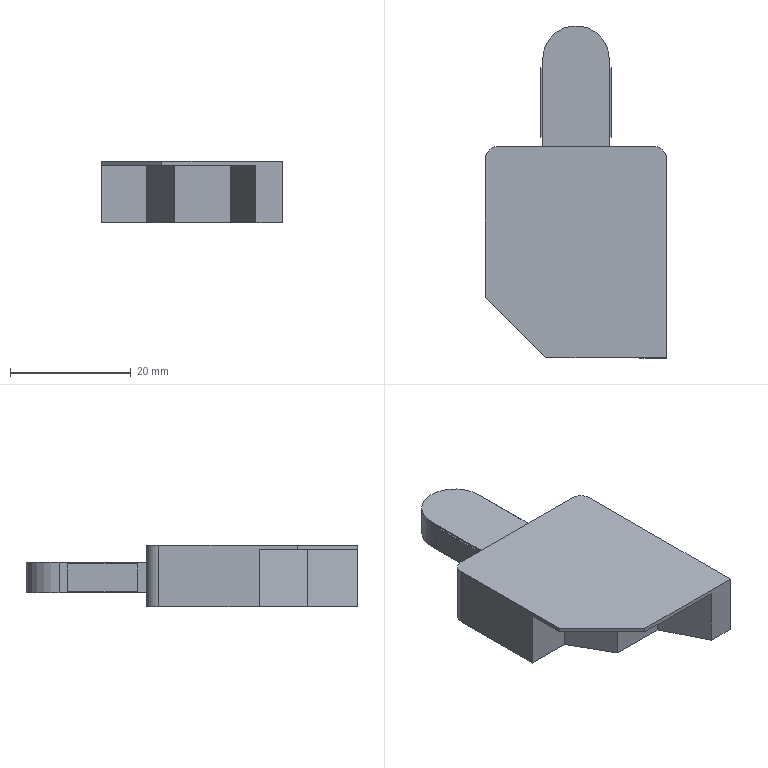Part | SolidWorks | features BaseBody 1 | 1 solid | 29 faces | box 30 x 55 x 10.2 mm | volume 9110 mm3 | plane 26 | cylinder 3 | commonest cylinder face diameters 4 x2 11 x1
STEP:
#1=CARTESIAN_POINT('',(244.946,-4065.971,2034.471));
#2=VERTEX_POINT('',#1);
#3=CARTESIAN_POINT('',(244.946,-4042.971,2034.471));
#4=VERTEX_POINT('',#3);
#5=CARTESIAN_POINT('',(244.946,-4075.971,2034.471));
#6=DIRECTION('',(0.,1.,0.));
#7=VECTOR('',#6,1000.);
#8=LINE('',#5,#7);
#9=EDGE_CURVE('',#2,#4,#8,.T.);
#10=ORIENTED_EDGE('',*,*,#9,.F.);
#11=CARTESIAN_POINT('',(254.946,-4075.971,2034.471));
#12=VERTEX_POINT('',#11);
#13=CARTESIAN_POINT('',(254.946,-4075.971,2034.471));
#14=DIRECTION('',(-0.7071,0.7071,0.));
#15=VECTOR('',#14,1000.);
#16=LINE('',#13,#15);
#17=EDGE_CURVE('',#12,#2,#16,.T.);
#18=ORIENTED_EDGE('',*,*,#17,.F.);
#19=CARTESIAN_POINT('',(274.946,-4075.971,2034.471));
#20=VERTEX_POINT('',#19);
#21=CARTESIAN_POINT('',(254.946,-4075.971,2034.471));
#22=DIRECTION('',(-1.,0.,0.));
#23=VECTOR('',#22,1000.);
#24=LINE('',#21,#23);
#25=EDGE_CURVE('',#20,#12,#24,.T.);
#26=ORIENTED_EDGE('',*,*,#25,.F.);
#27=CARTESIAN_POINT('',(274.946,-4042.971,2034.471));
#28=VERTEX_POINT('',#27);
#29=CARTESIAN_POINT('',(274.946,-4075.971,2034.471));
#30=DIRECTION('',(0.,-1.,0.));
#31=VECTOR('',#30,1000.);
#32=LINE('',#29,#31);
#33=EDGE_CURVE('',#28,#20,#32,.T.);
#34=ORIENTED_EDGE('',*,*,#33,.F.);
#35=CARTESIAN_POINT('',(272.946,-4040.971,2034.471));
#36=VERTEX_POINT('',#35);
#37=CARTESIAN_POINT('',(272.946,-4042.971,2034.471));
#38=DIRECTION('',(0.,0.,-1.));
#39=DIRECTION('',(1.,0.,0.));
#40=AXIS2_PLACEMENT_3D('',#37,#38,#39);
#41=CIRCLE('',#40,2.);
#42=EDGE_CURVE('',#36,#28,#41,.T.);
#43=ORIENTED_EDGE('',*,*,#42,.F.);
#44=CARTESIAN_POINT('',(246.946,-4040.971,2034.471));
#45=VERTEX_POINT('',#44);
#46=CARTESIAN_POINT('',(254.946,-4040.971,2034.471));
#47=DIRECTION('',(1.,0.,0.));
#48=VECTOR('',#47,1000.);
#49=LINE('',#46,#48);
#50=EDGE_CURVE('',#45,#36,#49,.T.);
#51=ORIENTED_EDGE('',*,*,#50,.F.);
#52=CARTESIAN_POINT('',(246.946,-4042.971,2034.471));
#53=DIRECTION('',(0.,0.,-1.));
#54=DIRECTION('',(1.,0.,0.));
#55=AXIS2_PLACEMENT_3D('',#52,#53,#54);
#56=CIRCLE('',#55,2.);
#57=EDGE_CURVE('',#4,#45,#56,.T.);
#58=ORIENTED_EDGE('',*,*,#57,.F.);
#59=EDGE_LOOP('',(#10,#18,#26,#34,#43,#51,#58));
#60=FACE_OUTER_BOUND('',#59,.T.);
#61=CARTESIAN_POINT('',(254.946,-4075.971,2034.471));
#62=DIRECTION('',(0.,0.,-1.));
#63=DIRECTION('',(-1.,0.,0.));
#64=AXIS2_PLACEMENT_3D('',#61,#62,#63);
#65=PLANE('',#64);
#66=ADVANCED_FACE('',(#60),#65,.F.);
#67=CARTESIAN_POINT('',(244.946,-4042.971,2024.271));
#68=VERTEX_POINT('',#67);
#69=CARTESIAN_POINT('',(244.946,-4042.971,2033.771));
#70=DIRECTION('',(0.,0.,1.));
#71=VECTOR('',#70,1000.);
#72=LINE('',#69,#71);
#73=EDGE_CURVE('',#68,#4,#72,.T.);
#74=ORIENTED_EDGE('',*,*,#73,.T.);
#75=ORIENTED_EDGE('',*,*,#57,.T.);
#76=CARTESIAN_POINT('',(246.946,-4040.971,2024.271));
#77=VERTEX_POINT('',#76);
#78=CARTESIAN_POINT('',(246.946,-4040.971,2033.771));
#79=DIRECTION('',(0.,0.,-1.));
#80=VECTOR('',#79,1000.);
#81=LINE('',#78,#80);
#82=EDGE_CURVE('',#45,#77,#81,.T.);
#83=ORIENTED_EDGE('',*,*,#82,.T.);
#84=CARTESIAN_POINT('',(246.946,-4042.971,2024.271));
#85=DIRECTION('',(0.,0.,1.));
#86=DIRECTION('',(1.,0.,0.));
#87=AXIS2_PLACEMENT_3D('',#84,#85,#86);
#88=CIRCLE('',#87,2.);
#89=EDGE_CURVE('',#77,#68,#88,.T.);
#90=ORIENTED_EDGE('',*,*,#89,.T.);
#91=EDGE_LOOP('',(#74,#75,#83,#90));
#92=FACE_OUTER_BOUND('',#91,.T.);
#93=CARTESIAN_POINT('',(246.946,-4042.971,2033.771));
#94=DIRECTION('',(0.,0.,1.));
#95=DIRECTION('',(1.,0.,0.));
#96=AXIS2_PLACEMENT_3D('',#93,#94,#95);
#97=CYLINDRICAL_SURFACE('',#96,2.);
#98=ADVANCED_FACE('',(#92),#97,.T.);
#99=CARTESIAN_POINT('',(244.946,-4065.971,2033.771));
#100=VERTEX_POINT('',#99);
#101=CARTESIAN_POINT('',(244.946,-4065.971,2033.771));
#102=DIRECTION('',(0.,0.,1.));
#103=VECTOR('',#102,1000.);
#104=LINE('',#101,#103);
#105=EDGE_CURVE('',#100,#2,#104,.T.);
#106=ORIENTED_EDGE('',*,*,#105,.T.);
#107=ORIENTED_EDGE('',*,*,#9,.T.);
#108=ORIENTED_EDGE('',*,*,#73,.F.);
#109=CARTESIAN_POINT('',(244.946,-4059.609,2024.271));
#110=VERTEX_POINT('',#109);
#111=CARTESIAN_POINT('',(244.946,-4065.971,2024.271));
#112=DIRECTION('',(0.,-1.,0.));
#113=VECTOR('',#112,1000.);
#114=LINE('',#111,#113);
#115=EDGE_CURVE('',#68,#110,#114,.T.);
#116=ORIENTED_EDGE('',*,*,#115,.T.);
#117=CARTESIAN_POINT('',(244.946,-4059.609,2033.771));
#118=VERTEX_POINT('',#117);
#119=CARTESIAN_POINT('',(244.946,-4059.609,2033.771));
#120=DIRECTION('',(0.,0.,1.));
#121=VECTOR('',#120,1000.);
#122=LINE('',#119,#121);
#123=EDGE_CURVE('',#110,#118,#122,.T.);
#124=ORIENTED_EDGE('',*,*,#123,.T.);
#125=CARTESIAN_POINT('',(244.946,-4065.971,2033.771));
#126=DIRECTION('',(0.,-1.,0.));
#127=VECTOR('',#126,1000.);
#128=LINE('',#125,#127);
#129=EDGE_CURVE('',#118,#100,#128,.T.);
#130=ORIENTED_EDGE('',*,*,#129,.T.);
#131=EDGE_LOOP('',(#106,#107,#108,#116,#124,#130));
#132=FACE_OUTER_BOUND('',#131,.T.);
#133=CARTESIAN_POINT('',(244.946,-4065.971,2033.771));
#134=DIRECTION('',(-1.,0.,0.));
#135=DIRECTION('',(0.,0.,1.));
#136=AXIS2_PLACEMENT_3D('',#133,#134,#135);
#137=PLANE('',#136);
#138=ADVANCED_FACE('',(#132),#137,.T.);
#139=CARTESIAN_POINT('',(254.946,-4075.971,2033.771));
#140=VERTEX_POINT('',#139);
#141=CARTESIAN_POINT('',(254.946,-4075.971,2033.771));
#142=DIRECTION('',(0.7071,-0.7071,0.));
#143=VECTOR('',#142,1000.);
#144=LINE('',#141,#143);
#145=EDGE_CURVE('',#100,#140,#144,.T.);
#146=ORIENTED_EDGE('',*,*,#145,.T.);
#147=CARTESIAN_POINT('',(254.946,-4075.971,2033.771));
#148=DIRECTION('',(0.,0.,1.));
#149=VECTOR('',#148,1000.);
#150=LINE('',#147,#149);
#151=EDGE_CURVE('',#140,#12,#150,.T.);
#152=ORIENTED_EDGE('',*,*,#151,.T.);
#153=ORIENTED_EDGE('',*,*,#17,.T.);
#154=ORIENTED_EDGE('',*,*,#105,.F.);
#155=EDGE_LOOP('',(#146,#152,#153,#154));
#156=FACE_OUTER_BOUND('',#155,.T.);
#157=CARTESIAN_POINT('',(254.946,-4075.971,2033.771));
#158=DIRECTION('',(-0.7071,-0.7071,0.));
#159=DIRECTION('',(0.7071,-0.7071,0.));
#160=AXIS2_PLACEMENT_3D('',#157,#158,#159);
#161=PLANE('',#160);
#162=ADVANCED_FACE('',(#156),#161,.T.);
#163=CARTESIAN_POINT('',(270.521,-4075.971,2024.271));
#164=VERTEX_POINT('',#163);
#165=CARTESIAN_POINT('',(274.946,-4075.971,2024.271));
#166=VERTEX_POINT('',#165);
#167=CARTESIAN_POINT('',(274.946,-4075.971,2024.271));
#168=DIRECTION('',(1.,0.,0.));
#169=VECTOR('',#168,1000.);
#170=LINE('',#167,#169);
#171=EDGE_CURVE('',#164,#166,#170,.T.);
#172=ORIENTED_EDGE('',*,*,#171,.T.);
#173=CARTESIAN_POINT('',(274.946,-4075.971,2033.771));
#174=DIRECTION('',(0.,0.,1.));
#175=VECTOR('',#174,1000.);
#176=LINE('',#173,#175);
#177=EDGE_CURVE('',#166,#20,#176,.T.);
#178=ORIENTED_EDGE('',*,*,#177,.T.);
#179=ORIENTED_EDGE('',*,*,#25,.T.);
#180=ORIENTED_EDGE('',*,*,#151,.F.);
#181=CARTESIAN_POINT('',(270.521,-4075.971,2033.771));
#182=VERTEX_POINT('',#181);
#183=CARTESIAN_POINT('',(274.946,-4075.971,2033.771));
#184=DIRECTION('',(1.,0.,0.));
#185=VECTOR('',#184,1000.);
#186=LINE('',#183,#185);
#187=EDGE_CURVE('',#140,#182,#186,.T.);
#188=ORIENTED_EDGE('',*,*,#187,.T.);
#189=CARTESIAN_POINT('',(270.521,-4075.971,2033.771));
#190=DIRECTION('',(0.,0.,-1.));
#191=VECTOR('',#190,1000.);
#192=LINE('',#189,#191);
#193=EDGE_CURVE('',#182,#164,#192,.T.);
#194=ORIENTED_EDGE('',*,*,#193,.T.);
#195=EDGE_LOOP('',(#172,#178,#179,#180,#188,#194));
#196=FACE_OUTER_BOUND('',#195,.T.);
#197=CARTESIAN_POINT('',(274.946,-4075.971,2033.771));
#198=DIRECTION('',(0.,-1.,0.));
#199=DIRECTION('',(0.,0.,-1.));
#200=AXIS2_PLACEMENT_3D('',#197,#198,#199);
#201=PLANE('',#200);
#202=ADVANCED_FACE('',(#196),#201,.T.);
#203=ORIENTED_EDGE('',*,*,#177,.F.);
#204=CARTESIAN_POINT('',(274.946,-4042.971,2024.271));
#205=VERTEX_POINT('',#204);
#206=CARTESIAN_POINT('',(274.946,-4040.971,2024.271));
#207=DIRECTION('',(0.,1.,0.));
#208=VECTOR('',#207,1000.);
#209=LINE('',#206,#208);
#210=EDGE_CURVE('',#166,#205,#209,.T.);
#211=ORIENTED_EDGE('',*,*,#210,.T.);
#212=CARTESIAN_POINT('',(274.946,-4042.971,2033.771));
#213=DIRECTION('',(0.,0.,1.));
#214=VECTOR('',#213,1000.);
#215=LINE('',#212,#214);
#216=EDGE_CURVE('',#205,#28,#215,.T.);
#217=ORIENTED_EDGE('',*,*,#216,.T.);
#218=ORIENTED_EDGE('',*,*,#33,.T.);
#219=EDGE_LOOP('',(#203,#211,#217,#218));
#220=FACE_OUTER_BOUND('',#219,.T.);
#221=CARTESIAN_POINT('',(274.946,-4040.971,2033.771));
#222=DIRECTION('',(1.,0.,0.));
#223=DIRECTION('',(0.,0.,-1.));
#224=AXIS2_PLACEMENT_3D('',#221,#222,#223);
#225=PLANE('',#224);
#226=ADVANCED_FACE('',(#220),#225,.T.);
#227=CARTESIAN_POINT('',(272.946,-4040.971,2024.271));
#228=VERTEX_POINT('',#227);
#229=CARTESIAN_POINT('',(272.946,-4040.971,2033.771));
#230=DIRECTION('',(0.,0.,1.));
#231=VECTOR('',#230,1000.);
#232=LINE('',#229,#231);
#233=EDGE_CURVE('',#228,#36,#232,.T.);
#234=ORIENTED_EDGE('',*,*,#233,.T.);
#235=ORIENTED_EDGE('',*,*,#42,.T.);
#236=ORIENTED_EDGE('',*,*,#216,.F.);
#237=CARTESIAN_POINT('',(272.946,-4042.971,2024.271));
#238=DIRECTION('',(0.,0.,1.));
#239=DIRECTION('',(1.,0.,0.));
#240=AXIS2_PLACEMENT_3D('',#237,#238,#239);
#241=CIRCLE('',#240,2.);
#242=EDGE_CURVE('',#205,#228,#241,.T.);
#243=ORIENTED_EDGE('',*,*,#242,.T.);
#244=EDGE_LOOP('',(#234,#235,#236,#243));
#245=FACE_OUTER_BOUND('',#244,.T.);
#246=CARTESIAN_POINT('',(272.946,-4042.971,2033.771));
#247=DIRECTION('',(0.,0.,1.));
#248=DIRECTION('',(1.,0.,0.));
#249=AXIS2_PLACEMENT_3D('',#246,#247,#248);
#250=CYLINDRICAL_SURFACE('',#249,2.);
#251=ADVANCED_FACE('',(#245),#250,.T.);
#252=ORIENTED_EDGE('',*,*,#233,.F.);
#253=CARTESIAN_POINT('',(244.946,-4040.971,2024.271));
#254=DIRECTION('',(-1.,0.,0.));
#255=VECTOR('',#254,1000.);
#256=LINE('',#253,#255);
#257=EDGE_CURVE('',#228,#77,#256,.T.);
#258=ORIENTED_EDGE('',*,*,#257,.T.);
#259=ORIENTED_EDGE('',*,*,#82,.F.);
#260=ORIENTED_EDGE('',*,*,#50,.T.);
#261=EDGE_LOOP('',(#252,#258,#259,#260));
#262=FACE_OUTER_BOUND('',#261,.T.);
#263=CARTESIAN_POINT('',(254.446,-4040.971,2031.613));
#264=VERTEX_POINT('',#263);
#265=CARTESIAN_POINT('',(254.446,-4040.971,2026.613));
#266=VERTEX_POINT('',#265);
#267=CARTESIAN_POINT('',(254.446,-4040.971,2033.771));
#268=DIRECTION('',(0.,0.,-1.));
#269=VECTOR('',#268,1000.);
#270=LINE('',#267,#269);
#271=EDGE_CURVE('',#264,#266,#270,.T.);
#272=ORIENTED_EDGE('',*,*,#271,.T.);
#273=CARTESIAN_POINT('',(265.446,-4040.971,2026.613));
#274=VERTEX_POINT('',#273);
#275=CARTESIAN_POINT('',(244.946,-4040.971,2026.613));
#276=DIRECTION('',(1.,0.,0.));
#277=VECTOR('',#276,1000.);
#278=LINE('',#275,#277);
#279=EDGE_CURVE('',#266,#274,#278,.T.);
#280=ORIENTED_EDGE('',*,*,#279,.T.);
#281=CARTESIAN_POINT('',(265.446,-4040.971,2031.613));
#282=VERTEX_POINT('',#281);
#283=CARTESIAN_POINT('',(265.446,-4040.971,2033.771));
#284=DIRECTION('',(0.,0.,1.));
#285=VECTOR('',#284,1000.);
#286=LINE('',#283,#285);
#287=EDGE_CURVE('',#274,#282,#286,.T.);
#288=ORIENTED_EDGE('',*,*,#287,.T.);
#289=CARTESIAN_POINT('',(244.946,-4040.971,2031.613));
#290=DIRECTION('',(-1.,0.,0.));
#291=VECTOR('',#290,1000.);
#292=LINE('',#289,#291);
#293=EDGE_CURVE('',#282,#264,#292,.T.);
#294=ORIENTED_EDGE('',*,*,#293,.T.);
#295=EDGE_LOOP('',(#272,#280,#288,#294));
#296=FACE_BOUND('',#295,.T.);
#297=CARTESIAN_POINT('',(244.946,-4040.971,2033.771));
#298=DIRECTION('',(0.,1.,0.));
#299=DIRECTION('',(0.,0.,1.));
#300=AXIS2_PLACEMENT_3D('',#297,#298,#299);
#301=PLANE('',#300);
#302=ADVANCED_FACE('',(#262,#296),#301,.T.);
#303=CARTESIAN_POINT('',(252.478,-4059.609,2024.271));
#304=VERTEX_POINT('',#303);
#305=CARTESIAN_POINT('',(260.766,-4059.609,2024.271));
#306=DIRECTION('',(-1.,0.,0.));
#307=VECTOR('',#306,1000.);
#308=LINE('',#305,#307);
#309=EDGE_CURVE('',#304,#110,#308,.T.);
#310=ORIENTED_EDGE('',*,*,#309,.T.);
#311=ORIENTED_EDGE('',*,*,#115,.F.);
#312=ORIENTED_EDGE('',*,*,#89,.F.);
#313=ORIENTED_EDGE('',*,*,#257,.F.);
#314=ORIENTED_EDGE('',*,*,#242,.F.);
#315=ORIENTED_EDGE('',*,*,#210,.F.);
#316=ORIENTED_EDGE('',*,*,#171,.F.);
#317=CARTESIAN_POINT('',(266.357,-4067.585,2024.271));
#318=VERTEX_POINT('',#317);
#319=CARTESIAN_POINT('',(270.521,-4075.971,2024.271));
#320=DIRECTION('',(-0.4447,0.8957,0.));
#321=VECTOR('',#320,1000.);
#322=LINE('',#319,#321);
#323=EDGE_CURVE('',#164,#318,#322,.T.);
#324=ORIENTED_EDGE('',*,*,#323,.T.);
#325=CARTESIAN_POINT('',(256.989,-4067.585,2024.271));
#326=VERTEX_POINT('',#325);
#327=CARTESIAN_POINT('',(260.766,-4067.585,2024.271));
#328=DIRECTION('',(-1.,0.,0.));
#329=VECTOR('',#328,1000.);
#330=LINE('',#327,#329);
#331=EDGE_CURVE('',#318,#326,#330,.T.);
#332=ORIENTED_EDGE('',*,*,#331,.T.);
#333=CARTESIAN_POINT('',(256.989,-4067.585,2024.271));
#334=DIRECTION('',(-0.4923,0.8704,0.));
#335=VECTOR('',#334,1000.);
#336=LINE('',#333,#335);
#337=EDGE_CURVE('',#326,#304,#336,.T.);
#338=ORIENTED_EDGE('',*,*,#337,.T.);
#339=EDGE_LOOP('',(#310,#311,#312,#313,#314,#315,#316,#324,#332,#338));
#340=FACE_OUTER_BOUND('',#339,.T.);
#341=CARTESIAN_POINT('',(260.766,-4061.034,2024.271));
#342=DIRECTION('',(0.,0.,-1.));
#343=DIRECTION('',(-1.,0.,0.));
#344=AXIS2_PLACEMENT_3D('',#341,#342,#343);
#345=PLANE('',#344);
#346=ADVANCED_FACE('',(#340),#345,.T.);
#347=ORIENTED_EDGE('',*,*,#145,.F.);
#348=ORIENTED_EDGE('',*,*,#129,.F.);
#349=CARTESIAN_POINT('',(252.478,-4059.609,2033.771));
#350=VERTEX_POINT('',#349);
#351=CARTESIAN_POINT('',(258.946,-4059.609,2033.771));
#352=DIRECTION('',(1.,0.,0.));
#353=VECTOR('',#352,1000.);
#354=LINE('',#351,#353);
#355=EDGE_CURVE('',#118,#350,#354,.T.);
#356=ORIENTED_EDGE('',*,*,#355,.T.);
#357=CARTESIAN_POINT('',(256.989,-4067.585,2033.771));
#358=VERTEX_POINT('',#357);
#359=CARTESIAN_POINT('',(252.478,-4059.609,2033.771));
#360=DIRECTION('',(0.4923,-0.8704,0.));
#361=VECTOR('',#360,1000.);
#362=LINE('',#359,#361);
#363=EDGE_CURVE('',#350,#358,#362,.T.);
#364=ORIENTED_EDGE('',*,*,#363,.T.);
#365=CARTESIAN_POINT('',(266.357,-4067.585,2033.771));
#366=VERTEX_POINT('',#365);
#367=CARTESIAN_POINT('',(258.946,-4067.585,2033.771));
#368=DIRECTION('',(1.,0.,0.));
#369=VECTOR('',#368,1000.);
#370=LINE('',#367,#369);
#371=EDGE_CURVE('',#358,#366,#370,.T.);
#372=ORIENTED_EDGE('',*,*,#371,.T.);
#373=CARTESIAN_POINT('',(266.357,-4067.585,2033.771));
#374=DIRECTION('',(0.4447,-0.8957,0.));
#375=VECTOR('',#374,1000.);
#376=LINE('',#373,#375);
#377=EDGE_CURVE('',#366,#182,#376,.T.);
#378=ORIENTED_EDGE('',*,*,#377,.T.);
#379=ORIENTED_EDGE('',*,*,#187,.F.);
#380=EDGE_LOOP('',(#347,#348,#356,#364,#372,#378,#379));
#381=FACE_OUTER_BOUND('',#380,.T.);
#382=CARTESIAN_POINT('',(258.946,-4059.971,2033.771));
#383=DIRECTION('',(0.,0.,-1.));
#384=DIRECTION('',(-1.,0.,0.));
#385=AXIS2_PLACEMENT_3D('',#382,#383,#384);
#386=PLANE('',#385);
#387=ADVANCED_FACE('',(#381),#386,.T.);
#388=ORIENTED_EDGE('',*,*,#309,.F.);
#389=CARTESIAN_POINT('',(252.478,-4059.609,2024.271));
#390=DIRECTION('',(0.,0.,1.));
#391=VECTOR('',#390,1000.);
#392=LINE('',#389,#391);
#393=EDGE_CURVE('',#304,#350,#392,.T.);
#394=ORIENTED_EDGE('',*,*,#393,.T.);
#395=ORIENTED_EDGE('',*,*,#355,.F.);
#396=ORIENTED_EDGE('',*,*,#123,.F.);
#397=EDGE_LOOP('',(#388,#394,#395,#396));
#398=FACE_OUTER_BOUND('',#397,.T.);
#399=CARTESIAN_POINT('',(252.478,-4059.609,2024.271));
#400=DIRECTION('',(0.,-1.,0.));
#401=DIRECTION('',(0.,0.,-1.));
#402=AXIS2_PLACEMENT_3D('',#399,#400,#401);
#403=PLANE('',#402);
#404=ADVANCED_FACE('',(#398),#403,.T.);
#405=ORIENTED_EDGE('',*,*,#323,.F.);
#406=ORIENTED_EDGE('',*,*,#193,.F.);
#407=ORIENTED_EDGE('',*,*,#377,.F.);
#408=CARTESIAN_POINT('',(266.357,-4067.585,2024.271));
#409=DIRECTION('',(0.,0.,-1.));
#410=VECTOR('',#409,1000.);
#411=LINE('',#408,#410);
#412=EDGE_CURVE('',#366,#318,#411,.T.);
#413=ORIENTED_EDGE('',*,*,#412,.T.);
#414=EDGE_LOOP('',(#405,#406,#407,#413));
#415=FACE_OUTER_BOUND('',#414,.T.);
#416=CARTESIAN_POINT('',(270.521,-4075.971,2024.271));
#417=DIRECTION('',(-0.8957,-0.4447,0.));
#418=DIRECTION('',(0.4447,-0.8957,0.));
#419=AXIS2_PLACEMENT_3D('',#416,#417,#418);
#420=PLANE('',#419);
#421=ADVANCED_FACE('',(#415),#420,.T.);
#422=CARTESIAN_POINT('',(265.446,-4026.471,2026.613));
#423=VERTEX_POINT('',#422);
#424=CARTESIAN_POINT('',(265.446,-4006.471,2026.613));
#425=DIRECTION('',(0.,1.,0.));
#426=VECTOR('',#425,1000.);
#427=LINE('',#424,#426);
#428=EDGE_CURVE('',#274,#423,#427,.T.);
#429=ORIENTED_EDGE('',*,*,#428,.F.);
#430=ORIENTED_EDGE('',*,*,#279,.F.);
#431=CARTESIAN_POINT('',(254.446,-4026.471,2026.613));
#432=VERTEX_POINT('',#431);
#433=CARTESIAN_POINT('',(254.446,-4006.471,2026.613));
#434=DIRECTION('',(0.,-1.,0.));
#435=VECTOR('',#434,1000.);
#436=LINE('',#433,#435);
#437=EDGE_CURVE('',#432,#266,#436,.T.);
#438=ORIENTED_EDGE('',*,*,#437,.F.);
#439=CARTESIAN_POINT('',(259.946,-4026.471,2026.613));
#440=DIRECTION('',(0.,0.,1.));
#441=DIRECTION('',(-1.,0.,0.));
#442=AXIS2_PLACEMENT_3D('',#439,#440,#441);
#443=CIRCLE('',#442,5.5);
#444=EDGE_CURVE('',#423,#432,#443,.T.);
#445=ORIENTED_EDGE('',*,*,#444,.F.);
#446=EDGE_LOOP('',(#429,#430,#438,#445));
#447=FACE_OUTER_BOUND('',#446,.T.);
#448=CARTESIAN_POINT('',(265.446,-4006.471,2026.613));
#449=DIRECTION('',(0.,0.,1.));
#450=DIRECTION('',(0.,-1.,0.));
#451=AXIS2_PLACEMENT_3D('',#448,#449,#450);
#452=PLANE('',#451);
#453=ADVANCED_FACE('',(#447),#452,.F.);
#454=CARTESIAN_POINT('',(254.446,-4027.908,2026.863));
#455=VERTEX_POINT('',#454);
#456=CARTESIAN_POINT('',(254.446,-4027.908,2031.363));
#457=VERTEX_POINT('',#456);
#458=CARTESIAN_POINT('',(254.446,-4027.908,2031.613));
#459=DIRECTION('',(0.,0.,1.));
#460=VECTOR('',#459,1000.);
#461=LINE('',#458,#460);
#462=EDGE_CURVE('',#455,#457,#461,.T.);
#463=ORIENTED_EDGE('',*,*,#462,.T.);
#464=CARTESIAN_POINT('',(254.446,-4039.428,2031.363));
#465=VERTEX_POINT('',#464);
#466=CARTESIAN_POINT('',(254.446,-4006.471,2031.363));
#467=DIRECTION('',(0.,-1.,0.));
#468=VECTOR('',#467,1000.);
#469=LINE('',#466,#468);
#470=EDGE_CURVE('',#457,#465,#469,.T.);
#471=ORIENTED_EDGE('',*,*,#470,.T.);
#472=CARTESIAN_POINT('',(254.446,-4039.428,2026.863));
#473=VERTEX_POINT('',#472);
#474=CARTESIAN_POINT('',(254.446,-4039.428,2031.613));
#475=DIRECTION('',(0.,0.,-1.));
#476=VECTOR('',#475,1000.);
#477=LINE('',#474,#476);
#478=EDGE_CURVE('',#465,#473,#477,.T.);
#479=ORIENTED_EDGE('',*,*,#478,.T.);
#480=CARTESIAN_POINT('',(254.446,-4006.471,2026.863));
#481=DIRECTION('',(0.,1.,0.));
#482=VECTOR('',#481,1000.);
#483=LINE('',#480,#482);
#484=EDGE_CURVE('',#473,#455,#483,.T.);
#485=ORIENTED_EDGE('',*,*,#484,.T.);
#486=EDGE_LOOP('',(#463,#471,#479,#485));
#487=FACE_BOUND('',#486,.T.);
#488=CARTESIAN_POINT('',(254.446,-4026.471,2031.613));
#489=VERTEX_POINT('',#488);
#490=CARTESIAN_POINT('',(254.446,-4006.471,2031.613));
#491=DIRECTION('',(0.,1.,0.));
#492=VECTOR('',#491,1000.);
#493=LINE('',#490,#492);
#494=EDGE_CURVE('',#264,#489,#493,.T.);
#495=ORIENTED_EDGE('',*,*,#494,.T.);
#496=CARTESIAN_POINT('',(254.446,-4026.471,2031.613));
#497=DIRECTION('',(0.,0.,-1.));
#498=VECTOR('',#497,1000.);
#499=LINE('',#496,#498);
#500=EDGE_CURVE('',#489,#432,#499,.T.);
#501=ORIENTED_EDGE('',*,*,#500,.T.);
#502=ORIENTED_EDGE('',*,*,#437,.T.);
#503=ORIENTED_EDGE('',*,*,#271,.F.);
#504=EDGE_LOOP('',(#495,#501,#502,#503));
#505=FACE_OUTER_BOUND('',#504,.T.);
#506=CARTESIAN_POINT('',(254.446,-4006.471,2031.613));
#507=DIRECTION('',(-1.,0.,0.));
#508=DIRECTION('',(0.,0.,1.));
#509=AXIS2_PLACEMENT_3D('',#506,#507,#508);
#510=PLANE('',#509);
#511=ADVANCED_FACE('',(#487,#505),#510,.T.);
#512=ORIENTED_EDGE('',*,*,#494,.F.);
#513=ORIENTED_EDGE('',*,*,#293,.F.);
#514=CARTESIAN_POINT('',(265.446,-4026.471,2031.613));
#515=VERTEX_POINT('',#514);
#516=CARTESIAN_POINT('',(265.446,-4014.431,2031.613));
#517=DIRECTION('',(0.,1.,0.));
#518=VECTOR('',#517,1000.);
#519=LINE('',#516,#518);
#520=EDGE_CURVE('',#282,#515,#519,.T.);
#521=ORIENTED_EDGE('',*,*,#520,.T.);
#522=CARTESIAN_POINT('',(259.946,-4026.471,2031.613));
#523=DIRECTION('',(0.,0.,1.));
#524=DIRECTION('',(-1.,0.,0.));
#525=AXIS2_PLACEMENT_3D('',#522,#523,#524);
#526=CIRCLE('',#525,5.5);
#527=EDGE_CURVE('',#515,#489,#526,.T.);
#528=ORIENTED_EDGE('',*,*,#527,.T.);
#529=EDGE_LOOP('',(#512,#513,#521,#528));
#530=FACE_OUTER_BOUND('',#529,.T.);
#531=CARTESIAN_POINT('',(259.946,-4014.431,2031.613));
#532=DIRECTION('',(0.,0.,1.));
#533=DIRECTION('',(0.,-1.,0.));
#534=AXIS2_PLACEMENT_3D('',#531,#532,#533);
#535=PLANE('',#534);
#536=ADVANCED_FACE('',(#530),#535,.T.);
#537=CARTESIAN_POINT('',(265.446,-4027.908,2031.363));
#538=VERTEX_POINT('',#537);
#539=CARTESIAN_POINT('',(265.446,-4027.908,2026.863));
#540=VERTEX_POINT('',#539);
#541=CARTESIAN_POINT('',(265.446,-4027.908,2031.613));
#542=DIRECTION('',(0.,0.,-1.));
#543=VECTOR('',#542,1000.);
#544=LINE('',#541,#543);
#545=EDGE_CURVE('',#538,#540,#544,.T.);
#546=ORIENTED_EDGE('',*,*,#545,.T.);
#547=CARTESIAN_POINT('',(265.446,-4039.428,2026.863));
#548=VERTEX_POINT('',#547);
#549=CARTESIAN_POINT('',(265.446,-4040.971,2026.863));
#550=DIRECTION('',(0.,-1.,0.));
#551=VECTOR('',#550,1000.);
#552=LINE('',#549,#551);
#553=EDGE_CURVE('',#540,#548,#552,.T.);
#554=ORIENTED_EDGE('',*,*,#553,.T.);
#555=CARTESIAN_POINT('',(265.446,-4039.428,2031.363));
#556=VERTEX_POINT('',#555);
#557=CARTESIAN_POINT('',(265.446,-4039.428,2031.613));
#558=DIRECTION('',(0.,0.,1.));
#559=VECTOR('',#558,1000.);
#560=LINE('',#557,#559);
#561=EDGE_CURVE('',#548,#556,#560,.T.);
#562=ORIENTED_EDGE('',*,*,#561,.T.);
#563=CARTESIAN_POINT('',(265.446,-4040.971,2031.363));
#564=DIRECTION('',(0.,1.,0.));
#565=VECTOR('',#564,1000.);
#566=LINE('',#563,#565);
#567=EDGE_CURVE('',#556,#538,#566,.T.);
#568=ORIENTED_EDGE('',*,*,#567,.T.);
#569=EDGE_LOOP('',(#546,#554,#562,#568));
#570=FACE_BOUND('',#569,.T.);
#571=ORIENTED_EDGE('',*,*,#520,.F.);
#572=ORIENTED_EDGE('',*,*,#287,.F.);
#573=ORIENTED_EDGE('',*,*,#428,.T.);
#574=CARTESIAN_POINT('',(265.446,-4026.471,2031.613));
#575=DIRECTION('',(0.,0.,1.));
#576=VECTOR('',#575,1000.);
#577=LINE('',#574,#576);
#578=EDGE_CURVE('',#423,#515,#577,.T.);
#579=ORIENTED_EDGE('',*,*,#578,.T.);
#580=EDGE_LOOP('',(#571,#572,#573,#579));
#581=FACE_OUTER_BOUND('',#580,.T.);
#582=CARTESIAN_POINT('',(265.446,-4040.971,2031.613));
#583=DIRECTION('',(1.,0.,0.));
#584=DIRECTION('',(0.,0.,-1.));
#585=AXIS2_PLACEMENT_3D('',#582,#583,#584);
#586=PLANE('',#585);
#587=ADVANCED_FACE('',(#570,#581),#586,.T.);
#588=ORIENTED_EDGE('',*,*,#337,.F.);
#589=CARTESIAN_POINT('',(256.989,-4067.585,2024.271));
#590=DIRECTION('',(0.,0.,1.));
#591=VECTOR('',#590,1000.);
#592=LINE('',#589,#591);
#593=EDGE_CURVE('',#326,#358,#592,.T.);
#594=ORIENTED_EDGE('',*,*,#593,.T.);
#595=ORIENTED_EDGE('',*,*,#363,.F.);
#596=ORIENTED_EDGE('',*,*,#393,.F.);
#597=EDGE_LOOP('',(#588,#594,#595,#596));
#598=FACE_OUTER_BOUND('',#597,.T.);
#599=CARTESIAN_POINT('',(256.989,-4067.585,2024.271));
#600=DIRECTION('',(-0.8704,-0.4923,0.));
#601=DIRECTION('',(0.4923,-0.8704,0.));
#602=AXIS2_PLACEMENT_3D('',#599,#600,#601);
#603=PLANE('',#602);
#604=ADVANCED_FACE('',(#598),#603,.T.);
#605=ORIENTED_EDGE('',*,*,#331,.F.);
#606=ORIENTED_EDGE('',*,*,#412,.F.);
#607=ORIENTED_EDGE('',*,*,#371,.F.);
#608=ORIENTED_EDGE('',*,*,#593,.F.);
#609=EDGE_LOOP('',(#605,#606,#607,#608));
#610=FACE_OUTER_BOUND('',#609,.T.);
#611=CARTESIAN_POINT('',(266.357,-4067.585,2024.271));
#612=DIRECTION('',(0.,-1.,0.));
#613=DIRECTION('',(0.,0.,-1.));
#614=AXIS2_PLACEMENT_3D('',#611,#612,#613);
#615=PLANE('',#614);
#616=ADVANCED_FACE('',(#610),#615,.T.);
#617=ORIENTED_EDGE('',*,*,#527,.F.);
#618=ORIENTED_EDGE('',*,*,#578,.F.);
#619=ORIENTED_EDGE('',*,*,#444,.T.);
#620=ORIENTED_EDGE('',*,*,#500,.F.);
#621=EDGE_LOOP('',(#617,#618,#619,#620));
#622=FACE_OUTER_BOUND('',#621,.T.);
#623=CARTESIAN_POINT('',(259.946,-4026.471,2031.613));
#624=DIRECTION('',(0.,0.,-1.));
#625=DIRECTION('',(-1.,0.,0.));
#626=AXIS2_PLACEMENT_3D('',#623,#624,#625);
#627=CYLINDRICAL_SURFACE('',#626,5.5);
#628=ADVANCED_FACE('',(#622),#627,.T.);
#629=CARTESIAN_POINT('',(254.146,-4027.908,2031.363));
#630=VERTEX_POINT('',#629);
#631=CARTESIAN_POINT('',(254.146,-4039.428,2031.363));
#632=VERTEX_POINT('',#631);
#633=CARTESIAN_POINT('',(254.146,-4023.668,2031.363));
#634=DIRECTION('',(0.,-1.,0.));
#635=VECTOR('',#634,1000.);
#636=LINE('',#633,#635);
#637=EDGE_CURVE('',#630,#632,#636,.T.);
#638=ORIENTED_EDGE('',*,*,#637,.T.);
#639=CARTESIAN_POINT('',(254.296,-4039.428,2031.363));
#640=DIRECTION('',(1.,0.,0.));
#641=VECTOR('',#640,1000.);
#642=LINE('',#639,#641);
#643=EDGE_CURVE('',#632,#465,#642,.T.);
#644=ORIENTED_EDGE('',*,*,#643,.T.);
#645=ORIENTED_EDGE('',*,*,#470,.F.);
#646=CARTESIAN_POINT('',(254.296,-4027.908,2031.363));
#647=DIRECTION('',(-1.,0.,0.));
#648=VECTOR('',#647,1000.);
#649=LINE('',#646,#648);
#650=EDGE_CURVE('',#457,#630,#649,.T.);
#651=ORIENTED_EDGE('',*,*,#650,.T.);
#652=EDGE_LOOP('',(#638,#644,#645,#651));
#653=FACE_OUTER_BOUND('',#652,.T.);
#654=CARTESIAN_POINT('',(254.296,-4023.668,2031.363));
#655=DIRECTION('',(0.,0.,1.));
#656=DIRECTION('',(0.,-1.,0.));
#657=AXIS2_PLACEMENT_3D('',#654,#655,#656);
#658=PLANE('',#657);
#659=ADVANCED_FACE('',(#653),#658,.T.);
#660=ORIENTED_EDGE('',*,*,#650,.F.);
#661=ORIENTED_EDGE('',*,*,#462,.F.);
#662=CARTESIAN_POINT('',(254.146,-4027.908,2026.863));
#663=VERTEX_POINT('',#662);
#664=CARTESIAN_POINT('',(254.446,-4027.908,2026.863));
#665=DIRECTION('',(-1.,0.,0.));
#666=VECTOR('',#665,1000.);
#667=LINE('',#664,#666);
#668=EDGE_CURVE('',#455,#663,#667,.T.);
#669=ORIENTED_EDGE('',*,*,#668,.T.);
#670=CARTESIAN_POINT('',(254.146,-4027.908,2031.363));
#671=DIRECTION('',(0.,0.,1.));
#672=VECTOR('',#671,1000.);
#673=LINE('',#670,#672);
#674=EDGE_CURVE('',#663,#630,#673,.T.);
#675=ORIENTED_EDGE('',*,*,#674,.T.);
#676=EDGE_LOOP('',(#660,#661,#669,#675));
#677=FACE_OUTER_BOUND('',#676,.T.);
#678=CARTESIAN_POINT('',(254.446,-4027.908,2031.363));
#679=DIRECTION('',(0.,1.,0.));
#680=DIRECTION('',(0.,0.,1.));
#681=AXIS2_PLACEMENT_3D('',#678,#679,#680);
#682=PLANE('',#681);
#683=ADVANCED_FACE('',(#677),#682,.T.);
#684=ORIENTED_EDGE('',*,*,#484,.F.);
#685=CARTESIAN_POINT('',(254.146,-4039.428,2026.863));
#686=VERTEX_POINT('',#685);
#687=CARTESIAN_POINT('',(254.446,-4039.428,2026.863));
#688=DIRECTION('',(1.,0.,0.));
#689=VECTOR('',#688,1000.);
#690=LINE('',#687,#689);
#691=EDGE_CURVE('',#686,#473,#690,.T.);
#692=ORIENTED_EDGE('',*,*,#691,.F.);
#693=CARTESIAN_POINT('',(254.146,-4007.908,2026.863));
#694=DIRECTION('',(0.,-1.,0.));
#695=VECTOR('',#694,1000.);
#696=LINE('',#693,#695);
#697=EDGE_CURVE('',#663,#686,#696,.T.);
#698=ORIENTED_EDGE('',*,*,#697,.F.);
#699=ORIENTED_EDGE('',*,*,#668,.F.);
#700=EDGE_LOOP('',(#684,#692,#698,#699));
#701=FACE_OUTER_BOUND('',#700,.T.);
#702=CARTESIAN_POINT('',(254.446,-4007.908,2026.863));
#703=DIRECTION('',(0.,0.,1.));
#704=DIRECTION('',(0.,-1.,0.));
#705=AXIS2_PLACEMENT_3D('',#702,#703,#704);
#706=PLANE('',#705);
#707=ADVANCED_FACE('',(#701),#706,.F.);
#708=ORIENTED_EDGE('',*,*,#643,.F.);
#709=CARTESIAN_POINT('',(254.146,-4039.428,2031.363));
#710=DIRECTION('',(0.,0.,-1.));
#711=VECTOR('',#710,1000.);
#712=LINE('',#709,#711);
#713=EDGE_CURVE('',#632,#686,#712,.T.);
#714=ORIENTED_EDGE('',*,*,#713,.T.);
#715=ORIENTED_EDGE('',*,*,#691,.T.);
#716=ORIENTED_EDGE('',*,*,#478,.F.);
#717=EDGE_LOOP('',(#708,#714,#715,#716));
#718=FACE_OUTER_BOUND('',#717,.T.);
#719=CARTESIAN_POINT('',(254.146,-4039.428,2031.363));
#720=DIRECTION('',(0.,-1.,0.));
#721=DIRECTION('',(0.,0.,-1.));
#722=AXIS2_PLACEMENT_3D('',#719,#720,#721);
#723=PLANE('',#722);
#724=ADVANCED_FACE('',(#718),#723,.T.);
#725=CARTESIAN_POINT('',(265.746,-4039.428,2026.863));
#726=VERTEX_POINT('',#725);
#727=CARTESIAN_POINT('',(265.746,-4027.908,2026.863));
#728=VERTEX_POINT('',#727);
#729=CARTESIAN_POINT('',(265.746,-4007.908,2026.863));
#730=DIRECTION('',(0.,1.,0.));
#731=VECTOR('',#730,1000.);
#732=LINE('',#729,#731);
#733=EDGE_CURVE('',#726,#728,#732,.T.);
#734=ORIENTED_EDGE('',*,*,#733,.F.);
#735=CARTESIAN_POINT('',(265.446,-4039.428,2026.863));
#736=DIRECTION('',(1.,0.,0.));
#737=VECTOR('',#736,1000.);
#738=LINE('',#735,#737);
#739=EDGE_CURVE('',#548,#726,#738,.T.);
#740=ORIENTED_EDGE('',*,*,#739,.F.);
#741=ORIENTED_EDGE('',*,*,#553,.F.);
#742=CARTESIAN_POINT('',(265.446,-4027.908,2026.863));
#743=DIRECTION('',(-1.,0.,0.));
#744=VECTOR('',#743,1000.);
#745=LINE('',#742,#744);
#746=EDGE_CURVE('',#728,#540,#745,.T.);
#747=ORIENTED_EDGE('',*,*,#746,.F.);
#748=EDGE_LOOP('',(#734,#740,#741,#747));
#749=FACE_OUTER_BOUND('',#748,.T.);
#750=CARTESIAN_POINT('',(265.446,-4007.908,2026.863));
#751=DIRECTION('',(0.,0.,1.));
#752=DIRECTION('',(0.,-1.,0.));
#753=AXIS2_PLACEMENT_3D('',#750,#751,#752);
#754=PLANE('',#753);
#755=ADVANCED_FACE('',(#749),#754,.F.);
#756=CARTESIAN_POINT('',(265.746,-4027.908,2031.363));
#757=VERTEX_POINT('',#756);
#758=CARTESIAN_POINT('',(265.446,-4027.908,2031.363));
#759=DIRECTION('',(1.,0.,0.));
#760=VECTOR('',#759,1000.);
#761=LINE('',#758,#760);
#762=EDGE_CURVE('',#538,#757,#761,.T.);
#763=ORIENTED_EDGE('',*,*,#762,.T.);
#764=CARTESIAN_POINT('',(265.746,-4027.908,2031.363));
#765=DIRECTION('',(0.,0.,-1.));
#766=VECTOR('',#765,1000.);
#767=LINE('',#764,#766);
#768=EDGE_CURVE('',#757,#728,#767,.T.);
#769=ORIENTED_EDGE('',*,*,#768,.T.);
#770=ORIENTED_EDGE('',*,*,#746,.T.);
#771=ORIENTED_EDGE('',*,*,#545,.F.);
#772=EDGE_LOOP('',(#763,#769,#770,#771));
#773=FACE_OUTER_BOUND('',#772,.T.);
#774=CARTESIAN_POINT('',(265.446,-4027.908,2031.363));
#775=DIRECTION('',(0.,1.,0.));
#776=DIRECTION('',(0.,0.,1.));
#777=AXIS2_PLACEMENT_3D('',#774,#775,#776);
#778=PLANE('',#777);
#779=ADVANCED_FACE('',(#773),#778,.T.);
#780=CARTESIAN_POINT('',(265.746,-4039.428,2031.363));
#781=VERTEX_POINT('',#780);
#782=CARTESIAN_POINT('',(265.746,-4023.668,2031.363));
#783=DIRECTION('',(0.,1.,0.));
#784=VECTOR('',#783,1000.);
#785=LINE('',#782,#784);
#786=EDGE_CURVE('',#781,#757,#785,.T.);
#787=ORIENTED_EDGE('',*,*,#786,.T.);
#788=ORIENTED_EDGE('',*,*,#762,.F.);
#789=ORIENTED_EDGE('',*,*,#567,.F.);
#790=CARTESIAN_POINT('',(265.596,-4039.428,2031.363));
#791=DIRECTION('',(1.,0.,0.));
#792=VECTOR('',#791,1000.);
#793=LINE('',#790,#792);
#794=EDGE_CURVE('',#556,#781,#793,.T.);
#795=ORIENTED_EDGE('',*,*,#794,.T.);
#796=EDGE_LOOP('',(#787,#788,#789,#795));
#797=FACE_OUTER_BOUND('',#796,.T.);
#798=CARTESIAN_POINT('',(265.596,-4023.668,2031.363));
#799=DIRECTION('',(0.,0.,1.));
#800=DIRECTION('',(0.,-1.,0.));
#801=AXIS2_PLACEMENT_3D('',#798,#799,#800);
#802=PLANE('',#801);
#803=ADVANCED_FACE('',(#797),#802,.T.);
#804=ORIENTED_EDGE('',*,*,#794,.F.);
#805=ORIENTED_EDGE('',*,*,#561,.F.);
#806=ORIENTED_EDGE('',*,*,#739,.T.);
#807=CARTESIAN_POINT('',(265.746,-4039.428,2031.363));
#808=DIRECTION('',(0.,0.,1.));
#809=VECTOR('',#808,1000.);
#810=LINE('',#807,#809);
#811=EDGE_CURVE('',#726,#781,#810,.T.);
#812=ORIENTED_EDGE('',*,*,#811,.T.);
#813=EDGE_LOOP('',(#804,#805,#806,#812));
#814=FACE_OUTER_BOUND('',#813,.T.);
#815=CARTESIAN_POINT('',(265.746,-4039.428,2031.363));
#816=DIRECTION('',(0.,-1.,0.));
#817=DIRECTION('',(0.,0.,-1.));
#818=AXIS2_PLACEMENT_3D('',#815,#816,#817);
#819=PLANE('',#818);
#820=ADVANCED_FACE('',(#814),#819,.T.);
#821=ORIENTED_EDGE('',*,*,#637,.F.);
#822=ORIENTED_EDGE('',*,*,#674,.F.);
#823=ORIENTED_EDGE('',*,*,#697,.T.);
#824=ORIENTED_EDGE('',*,*,#713,.F.);
#825=EDGE_LOOP('',(#821,#822,#823,#824));
#826=FACE_OUTER_BOUND('',#825,.T.);
#827=CARTESIAN_POINT('',(254.146,-4007.908,2031.363));
#828=DIRECTION('',(-1.,0.,0.));
#829=DIRECTION('',(0.,0.,1.));
#830=AXIS2_PLACEMENT_3D('',#827,#828,#829);
#831=PLANE('',#830);
#832=ADVANCED_FACE('',(#826),#831,.T.);
#833=ORIENTED_EDGE('',*,*,#786,.F.);
#834=ORIENTED_EDGE('',*,*,#811,.F.);
#835=ORIENTED_EDGE('',*,*,#733,.T.);
#836=ORIENTED_EDGE('',*,*,#768,.F.);
#837=EDGE_LOOP('',(#833,#834,#835,#836));
#838=FACE_OUTER_BOUND('',#837,.T.);
#839=CARTESIAN_POINT('',(265.746,-4027.908,2031.363));
#840=DIRECTION('',(1.,0.,0.));
#841=DIRECTION('',(0.,0.,-1.));
#842=AXIS2_PLACEMENT_3D('',#839,#840,#841);
#843=PLANE('',#842);
#844=ADVANCED_FACE('',(#838),#843,.T.);
#845=CLOSED_SHELL('',(#66,#98,#138,#162,#202,#226,#251,#302,#346,#387,#404,#421,#453,#511,#536,#587,#604,#616,#628,#659,#683,#707,#724,#755,#779,#803,#820,#832,#844));
#846=MANIFOLD_SOLID_BREP('',#845);
#847=CARTESIAN_POINT('',(0.,0.,0.));
#848=DIRECTION('',(0.,0.,1.));
#849=DIRECTION('',(1.,0.,0.));
#850=AXIS2_PLACEMENT_3D('',#847,#848,#849);
#851=(LENGTH_UNIT()NAMED_UNIT(*)SI_UNIT(.MILLI.,.METRE.));
#852=UNCERTAINTY_MEASURE_WITH_UNIT(LENGTH_MEASURE(0.00001),#851,'','');
#853=(NAMED_UNIT(*)PLANE_ANGLE_UNIT()SI_UNIT($,.RADIAN.));
#854=(NAMED_UNIT(*)SI_UNIT($,.STERADIAN.)SOLID_ANGLE_UNIT());
#855=(GEOMETRIC_REPRESENTATION_CONTEXT(3)GLOBAL_UNCERTAINTY_ASSIGNED_CONTEXT((#852))GLOBAL_UNIT_ASSIGNED_CONTEXT((#851,#853,#854))REPRESENTATION_CONTEXT('',''));
#856=ADVANCED_BREP_SHAPE_REPRESENTATION('',(#846,#850),#855);